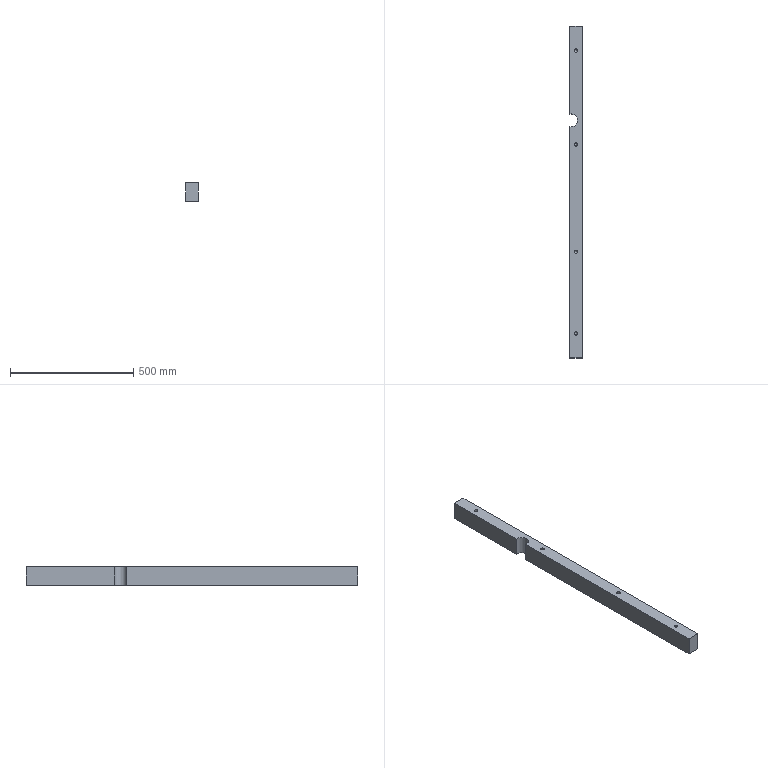Part | NX | features 3 2 | 1 solid | 24 faces | box 50 x 1345 x 75.5 mm | volume 4964830 mm3 | cylinder 9 | cone 8 | plane 7 | commonest cylinder face diameters 14.1 x8 52 x1
STEP:
#1=CARTESIAN_POINT('',(347.05,-572.5,256.5));
#2=VERTEX_POINT('',#1);
#3=CARTESIAN_POINT('',(340.,-572.5,256.5));
#4=DIRECTION('',(0.,0.,-1.));
#5=DIRECTION('',(1.,0.,0.));
#6=AXIS2_PLACEMENT_3D('',#3,#4,#5);
#7=CIRCLE('',#6,7.05);
#8=EDGE_CURVE('',#2,#2,#7,.T.);
#9=ORIENTED_EDGE('',*,*,#8,.T.);
#10=EDGE_LOOP('',(#9));
#11=FACE_BOUND('',#10,.T.);
#12=CARTESIAN_POINT('',(347.05,192.5,256.5));
#13=VERTEX_POINT('',#12);
#14=CARTESIAN_POINT('',(340.,192.5,256.5));
#15=DIRECTION('',(0.,0.,-1.));
#16=DIRECTION('',(1.,0.,0.));
#17=AXIS2_PLACEMENT_3D('',#14,#15,#16);
#18=CIRCLE('',#17,7.05);
#19=EDGE_CURVE('',#13,#13,#18,.T.);
#20=ORIENTED_EDGE('',*,*,#19,.T.);
#21=EDGE_LOOP('',(#20));
#22=FACE_BOUND('',#21,.T.);
#23=CARTESIAN_POINT('',(315.,315.515,256.5));
#24=VERTEX_POINT('',#23);
#25=CARTESIAN_POINT('',(315.,672.5,256.5));
#26=VERTEX_POINT('',#25);
#27=CARTESIAN_POINT('',(315.,193.,256.5));
#28=DIRECTION('',(0.,1.,0.));
#29=VECTOR('',#28,1000.);
#30=LINE('',#27,#29);
#31=EDGE_CURVE('',#24,#26,#30,.T.);
#32=ORIENTED_EDGE('',*,*,#31,.F.);
#33=CARTESIAN_POINT('',(315.,264.485,256.5));
#34=VERTEX_POINT('',#33);
#35=CARTESIAN_POINT('',(320.,290.,256.5));
#36=DIRECTION('',(0.,0.,1.));
#37=DIRECTION('',(1.,0.,0.));
#38=AXIS2_PLACEMENT_3D('',#35,#36,#37);
#39=CIRCLE('',#38,26.);
#40=EDGE_CURVE('',#34,#24,#39,.T.);
#41=ORIENTED_EDGE('',*,*,#40,.F.);
#42=CARTESIAN_POINT('',(315.,-672.5,256.5));
#43=VERTEX_POINT('',#42);
#44=CARTESIAN_POINT('',(315.,193.,256.5));
#45=DIRECTION('',(0.,1.,0.));
#46=VECTOR('',#45,1000.);
#47=LINE('',#44,#46);
#48=EDGE_CURVE('',#43,#34,#47,.T.);
#49=ORIENTED_EDGE('',*,*,#48,.F.);
#50=CARTESIAN_POINT('',(365.,-672.5,256.5));
#51=VERTEX_POINT('',#50);
#52=CARTESIAN_POINT('',(292.5,-672.5,256.5));
#53=DIRECTION('',(-1.,0.,0.));
#54=VECTOR('',#53,1000.);
#55=LINE('',#52,#54);
#56=EDGE_CURVE('',#51,#43,#55,.T.);
#57=ORIENTED_EDGE('',*,*,#56,.F.);
#58=CARTESIAN_POINT('',(365.,672.5,256.5));
#59=VERTEX_POINT('',#58);
#60=CARTESIAN_POINT('',(365.,193.,256.5));
#61=DIRECTION('',(0.,-1.,0.));
#62=VECTOR('',#61,1000.);
#63=LINE('',#60,#62);
#64=EDGE_CURVE('',#59,#51,#63,.T.);
#65=ORIENTED_EDGE('',*,*,#64,.F.);
#66=CARTESIAN_POINT('',(315.,672.5,256.5));
#67=DIRECTION('',(1.,0.,0.));
#68=VECTOR('',#67,1000.);
#69=LINE('',#66,#68);
#70=EDGE_CURVE('',#26,#59,#69,.T.);
#71=ORIENTED_EDGE('',*,*,#70,.F.);
#72=EDGE_LOOP('',(#32,#41,#49,#57,#65,#71));
#73=FACE_BOUND('',#72,.T.);
#74=CARTESIAN_POINT('',(347.05,572.5,256.5));
#75=VERTEX_POINT('',#74);
#76=CARTESIAN_POINT('',(340.,572.5,256.5));
#77=DIRECTION('',(0.,0.,-1.));
#78=DIRECTION('',(1.,0.,0.));
#79=AXIS2_PLACEMENT_3D('',#76,#77,#78);
#80=CIRCLE('',#79,7.05);
#81=EDGE_CURVE('',#75,#75,#80,.T.);
#82=ORIENTED_EDGE('',*,*,#81,.T.);
#83=EDGE_LOOP('',(#82));
#84=FACE_BOUND('',#83,.T.);
#85=CARTESIAN_POINT('',(347.05,-242.5,256.5));
#86=VERTEX_POINT('',#85);
#87=CARTESIAN_POINT('',(340.,-242.5,256.5));
#88=DIRECTION('',(0.,0.,-1.));
#89=DIRECTION('',(1.,0.,0.));
#90=AXIS2_PLACEMENT_3D('',#87,#88,#89);
#91=CIRCLE('',#90,7.05);
#92=EDGE_CURVE('',#86,#86,#91,.T.);
#93=ORIENTED_EDGE('',*,*,#92,.T.);
#94=EDGE_LOOP('',(#93));
#95=FACE_BOUND('',#94,.T.);
#96=CARTESIAN_POINT('',(2355.,0.,256.5));
#97=DIRECTION('',(0.,0.,1.));
#98=DIRECTION('',(-1.,0.,0.));
#99=AXIS2_PLACEMENT_3D('',#96,#97,#98);
#100=PLANE('',#99);
#101=ADVANCED_FACE('',(#11,#22,#73,#84,#95),#100,.T.);
#102=CARTESIAN_POINT('',(347.05,572.5,181.));
#103=VERTEX_POINT('',#102);
#104=CARTESIAN_POINT('',(340.,572.5,181.));
#105=DIRECTION('',(0.,0.,1.));
#106=DIRECTION('',(1.,0.,0.));
#107=AXIS2_PLACEMENT_3D('',#104,#105,#106);
#108=CIRCLE('',#107,7.05);
#109=EDGE_CURVE('',#103,#103,#108,.T.);
#110=ORIENTED_EDGE('',*,*,#109,.T.);
#111=EDGE_LOOP('',(#110));
#112=FACE_BOUND('',#111,.T.);
#113=CARTESIAN_POINT('',(347.05,-242.5,181.));
#114=VERTEX_POINT('',#113);
#115=CARTESIAN_POINT('',(340.,-242.5,181.));
#116=DIRECTION('',(0.,0.,1.));
#117=DIRECTION('',(1.,0.,0.));
#118=AXIS2_PLACEMENT_3D('',#115,#116,#117);
#119=CIRCLE('',#118,7.05);
#120=EDGE_CURVE('',#114,#114,#119,.T.);
#121=ORIENTED_EDGE('',*,*,#120,.T.);
#122=EDGE_LOOP('',(#121));
#123=FACE_BOUND('',#122,.T.);
#124=CARTESIAN_POINT('',(315.,264.485,181.));
#125=VERTEX_POINT('',#124);
#126=CARTESIAN_POINT('',(315.,-672.5,181.));
#127=VERTEX_POINT('',#126);
#128=CARTESIAN_POINT('',(315.,193.,181.));
#129=DIRECTION('',(0.,-1.,0.));
#130=VECTOR('',#129,1000.);
#131=LINE('',#128,#130);
#132=EDGE_CURVE('',#125,#127,#131,.T.);
#133=ORIENTED_EDGE('',*,*,#132,.F.);
#134=CARTESIAN_POINT('',(315.,315.515,181.));
#135=VERTEX_POINT('',#134);
#136=CARTESIAN_POINT('',(320.,290.,181.));
#137=DIRECTION('',(0.,0.,-1.));
#138=DIRECTION('',(-1.,0.,0.));
#139=AXIS2_PLACEMENT_3D('',#136,#137,#138);
#140=CIRCLE('',#139,26.);
#141=EDGE_CURVE('',#135,#125,#140,.T.);
#142=ORIENTED_EDGE('',*,*,#141,.F.);
#143=CARTESIAN_POINT('',(315.,672.5,181.));
#144=VERTEX_POINT('',#143);
#145=CARTESIAN_POINT('',(315.,193.,181.));
#146=DIRECTION('',(0.,-1.,0.));
#147=VECTOR('',#146,1000.);
#148=LINE('',#145,#147);
#149=EDGE_CURVE('',#144,#135,#148,.T.);
#150=ORIENTED_EDGE('',*,*,#149,.F.);
#151=CARTESIAN_POINT('',(365.,672.5,181.));
#152=VERTEX_POINT('',#151);
#153=CARTESIAN_POINT('',(1585.,672.5,181.));
#154=DIRECTION('',(1.,0.,0.));
#155=VECTOR('',#154,1000.);
#156=LINE('',#153,#155);
#157=EDGE_CURVE('',#144,#152,#156,.T.);
#158=ORIENTED_EDGE('',*,*,#157,.T.);
#159=CARTESIAN_POINT('',(365.,-672.5,181.));
#160=VERTEX_POINT('',#159);
#161=CARTESIAN_POINT('',(365.,193.,181.));
#162=DIRECTION('',(0.,1.,0.));
#163=VECTOR('',#162,1000.);
#164=LINE('',#161,#163);
#165=EDGE_CURVE('',#160,#152,#164,.T.);
#166=ORIENTED_EDGE('',*,*,#165,.F.);
#167=CARTESIAN_POINT('',(1585.,-672.5,181.));
#168=DIRECTION('',(-1.,0.,0.));
#169=VECTOR('',#168,1000.);
#170=LINE('',#167,#169);
#171=EDGE_CURVE('',#160,#127,#170,.T.);
#172=ORIENTED_EDGE('',*,*,#171,.T.);
#173=EDGE_LOOP('',(#133,#142,#150,#158,#166,#172));
#174=FACE_BOUND('',#173,.T.);
#175=CARTESIAN_POINT('',(347.05,-572.5,181.));
#176=VERTEX_POINT('',#175);
#177=CARTESIAN_POINT('',(340.,-572.5,181.));
#178=DIRECTION('',(0.,0.,1.));
#179=DIRECTION('',(1.,0.,0.));
#180=AXIS2_PLACEMENT_3D('',#177,#178,#179);
#181=CIRCLE('',#180,7.05);
#182=EDGE_CURVE('',#176,#176,#181,.T.);
#183=ORIENTED_EDGE('',*,*,#182,.T.);
#184=EDGE_LOOP('',(#183));
#185=FACE_BOUND('',#184,.T.);
#186=CARTESIAN_POINT('',(347.05,192.5,181.));
#187=VERTEX_POINT('',#186);
#188=CARTESIAN_POINT('',(340.,192.5,181.));
#189=DIRECTION('',(0.,0.,1.));
#190=DIRECTION('',(1.,0.,0.));
#191=AXIS2_PLACEMENT_3D('',#188,#189,#190);
#192=CIRCLE('',#191,7.05);
#193=EDGE_CURVE('',#187,#187,#192,.T.);
#194=ORIENTED_EDGE('',*,*,#193,.T.);
#195=EDGE_LOOP('',(#194));
#196=FACE_BOUND('',#195,.T.);
#197=CARTESIAN_POINT('',(1585.,193.,181.));
#198=DIRECTION('',(0.,0.,-1.));
#199=DIRECTION('',(-1.,0.,0.));
#200=AXIS2_PLACEMENT_3D('',#197,#198,#199);
#201=PLANE('',#200);
#202=ADVANCED_FACE('',(#112,#123,#174,#185,#196),#201,.T.);
#203=ORIENTED_EDGE('',*,*,#48,.T.);
#204=CARTESIAN_POINT('',(315.,264.485,218.75));
#205=DIRECTION('',(0.,0.,-1.));
#206=VECTOR('',#205,1000.);
#207=LINE('',#204,#206);
#208=EDGE_CURVE('',#34,#125,#207,.T.);
#209=ORIENTED_EDGE('',*,*,#208,.T.);
#210=ORIENTED_EDGE('',*,*,#132,.T.);
#211=CARTESIAN_POINT('',(315.,-672.5,-1.5));
#212=DIRECTION('',(0.,0.,1.));
#213=VECTOR('',#212,1000.);
#214=LINE('',#211,#213);
#215=EDGE_CURVE('',#127,#43,#214,.T.);
#216=ORIENTED_EDGE('',*,*,#215,.T.);
#217=EDGE_LOOP('',(#203,#209,#210,#216));
#218=FACE_BOUND('',#217,.T.);
#219=CARTESIAN_POINT('',(315.,193.,-1.5));
#220=DIRECTION('',(-1.,0.,0.));
#221=DIRECTION('',(0.,0.,-1.));
#222=AXIS2_PLACEMENT_3D('',#219,#220,#221);
#223=PLANE('',#222);
#224=ADVANCED_FACE('',(#218),#223,.T.);
#225=ORIENTED_EDGE('',*,*,#149,.T.);
#226=CARTESIAN_POINT('',(315.,315.515,218.75));
#227=DIRECTION('',(0.,0.,1.));
#228=VECTOR('',#227,1000.);
#229=LINE('',#226,#228);
#230=EDGE_CURVE('',#135,#24,#229,.T.);
#231=ORIENTED_EDGE('',*,*,#230,.T.);
#232=ORIENTED_EDGE('',*,*,#31,.T.);
#233=CARTESIAN_POINT('',(315.,672.5,-1.5));
#234=DIRECTION('',(0.,0.,-1.));
#235=VECTOR('',#234,1000.);
#236=LINE('',#233,#235);
#237=EDGE_CURVE('',#26,#144,#236,.T.);
#238=ORIENTED_EDGE('',*,*,#237,.T.);
#239=EDGE_LOOP('',(#225,#231,#232,#238));
#240=FACE_BOUND('',#239,.T.);
#241=CARTESIAN_POINT('',(315.,193.,-1.5));
#242=DIRECTION('',(-1.,0.,0.));
#243=DIRECTION('',(0.,0.,-1.));
#244=AXIS2_PLACEMENT_3D('',#241,#242,#243);
#245=PLANE('',#244);
#246=ADVANCED_FACE('',(#240),#245,.T.);
#247=CARTESIAN_POINT('',(365.,672.5,-1.5));
#248=DIRECTION('',(0.,0.,1.));
#249=VECTOR('',#248,1000.);
#250=LINE('',#247,#249);
#251=EDGE_CURVE('',#152,#59,#250,.T.);
#252=ORIENTED_EDGE('',*,*,#251,.T.);
#253=ORIENTED_EDGE('',*,*,#64,.T.);
#254=CARTESIAN_POINT('',(365.,-672.5,-1.5));
#255=DIRECTION('',(0.,0.,-1.));
#256=VECTOR('',#255,1000.);
#257=LINE('',#254,#256);
#258=EDGE_CURVE('',#51,#160,#257,.T.);
#259=ORIENTED_EDGE('',*,*,#258,.T.);
#260=ORIENTED_EDGE('',*,*,#165,.T.);
#261=EDGE_LOOP('',(#252,#253,#259,#260));
#262=FACE_BOUND('',#261,.T.);
#263=CARTESIAN_POINT('',(365.,193.,-1.5));
#264=DIRECTION('',(1.,0.,0.));
#265=DIRECTION('',(0.,0.,1.));
#266=AXIS2_PLACEMENT_3D('',#263,#264,#265);
#267=PLANE('',#266);
#268=ADVANCED_FACE('',(#262),#267,.T.);
#269=ORIENTED_EDGE('',*,*,#258,.F.);
#270=ORIENTED_EDGE('',*,*,#56,.T.);
#271=ORIENTED_EDGE('',*,*,#215,.F.);
#272=ORIENTED_EDGE('',*,*,#171,.F.);
#273=EDGE_LOOP('',(#269,#270,#271,#272));
#274=FACE_BOUND('',#273,.T.);
#275=CARTESIAN_POINT('',(292.5,-672.5,-103.));
#276=DIRECTION('',(0.,1.,0.));
#277=DIRECTION('',(1.,0.,0.));
#278=AXIS2_PLACEMENT_3D('',#275,#276,#277);
#279=PLANE('',#278);
#280=ADVANCED_FACE('',(#274),#279,.F.);
#281=ORIENTED_EDGE('',*,*,#237,.F.);
#282=ORIENTED_EDGE('',*,*,#70,.T.);
#283=ORIENTED_EDGE('',*,*,#251,.F.);
#284=ORIENTED_EDGE('',*,*,#157,.F.);
#285=EDGE_LOOP('',(#281,#282,#283,#284));
#286=FACE_BOUND('',#285,.T.);
#287=CARTESIAN_POINT('',(315.,672.5,231.5));
#288=DIRECTION('',(0.,1.,0.));
#289=DIRECTION('',(0.,0.,-1.));
#290=AXIS2_PLACEMENT_3D('',#287,#288,#289);
#291=PLANE('',#290);
#292=ADVANCED_FACE('',(#286),#291,.T.);
#293=ORIENTED_EDGE('',*,*,#40,.T.);
#294=ORIENTED_EDGE('',*,*,#230,.F.);
#295=ORIENTED_EDGE('',*,*,#141,.T.);
#296=ORIENTED_EDGE('',*,*,#208,.F.);
#297=EDGE_LOOP('',(#293,#294,#295,#296));
#298=FACE_BOUND('',#297,.T.);
#299=CARTESIAN_POINT('',(320.,290.,-261.5));
#300=DIRECTION('',(0.,0.,1.));
#301=DIRECTION('',(-1.,0.,0.));
#302=AXIS2_PLACEMENT_3D('',#299,#300,#301);
#303=CYLINDRICAL_SURFACE('',#302,26.);
#304=ADVANCED_FACE('',(#298),#303,.F.);
#305=ORIENTED_EDGE('',*,*,#120,.F.);
#306=EDGE_LOOP('',(#305));
#307=FACE_BOUND('',#306,.T.);
#308=CARTESIAN_POINT('',(347.05,-242.5,188.95));
#309=VERTEX_POINT('',#308);
#310=CARTESIAN_POINT('',(340.,-242.5,188.95));
#311=DIRECTION('',(0.,0.,-1.));
#312=DIRECTION('',(1.,0.,0.));
#313=AXIS2_PLACEMENT_3D('',#310,#311,#312);
#314=CIRCLE('',#313,7.05);
#315=EDGE_CURVE('',#309,#309,#314,.T.);
#316=ORIENTED_EDGE('',*,*,#315,.F.);
#317=EDGE_LOOP('',(#316));
#318=FACE_BOUND('',#317,.T.);
#319=CARTESIAN_POINT('',(340.,-242.5,181.));
#320=DIRECTION('',(0.,0.,1.));
#321=DIRECTION('',(-1.,0.,0.));
#322=AXIS2_PLACEMENT_3D('',#319,#320,#321);
#323=CYLINDRICAL_SURFACE('',#322,7.05);
#324=ADVANCED_FACE('',(#307,#318),#323,.F.);
#325=ORIENTED_EDGE('',*,*,#182,.F.);
#326=EDGE_LOOP('',(#325));
#327=FACE_BOUND('',#326,.T.);
#328=CARTESIAN_POINT('',(347.05,-572.5,188.95));
#329=VERTEX_POINT('',#328);
#330=CARTESIAN_POINT('',(340.,-572.5,188.95));
#331=DIRECTION('',(0.,0.,-1.));
#332=DIRECTION('',(1.,0.,0.));
#333=AXIS2_PLACEMENT_3D('',#330,#331,#332);
#334=CIRCLE('',#333,7.05);
#335=EDGE_CURVE('',#329,#329,#334,.T.);
#336=ORIENTED_EDGE('',*,*,#335,.F.);
#337=EDGE_LOOP('',(#336));
#338=FACE_BOUND('',#337,.T.);
#339=CARTESIAN_POINT('',(340.,-572.5,181.));
#340=DIRECTION('',(0.,0.,1.));
#341=DIRECTION('',(-1.,0.,0.));
#342=AXIS2_PLACEMENT_3D('',#339,#340,#341);
#343=CYLINDRICAL_SURFACE('',#342,7.05);
#344=ADVANCED_FACE('',(#327,#338),#343,.F.);
#345=ORIENTED_EDGE('',*,*,#109,.F.);
#346=EDGE_LOOP('',(#345));
#347=FACE_BOUND('',#346,.T.);
#348=CARTESIAN_POINT('',(347.05,572.5,188.95));
#349=VERTEX_POINT('',#348);
#350=CARTESIAN_POINT('',(340.,572.5,188.95));
#351=DIRECTION('',(0.,0.,-1.));
#352=DIRECTION('',(1.,0.,0.));
#353=AXIS2_PLACEMENT_3D('',#350,#351,#352);
#354=CIRCLE('',#353,7.05);
#355=EDGE_CURVE('',#349,#349,#354,.T.);
#356=ORIENTED_EDGE('',*,*,#355,.F.);
#357=EDGE_LOOP('',(#356));
#358=FACE_BOUND('',#357,.T.);
#359=CARTESIAN_POINT('',(340.,572.5,181.));
#360=DIRECTION('',(0.,0.,1.));
#361=DIRECTION('',(-1.,0.,0.));
#362=AXIS2_PLACEMENT_3D('',#359,#360,#361);
#363=CYLINDRICAL_SURFACE('',#362,7.05);
#364=ADVANCED_FACE('',(#347,#358),#363,.F.);
#365=ORIENTED_EDGE('',*,*,#193,.F.);
#366=EDGE_LOOP('',(#365));
#367=FACE_BOUND('',#366,.T.);
#368=CARTESIAN_POINT('',(347.05,192.5,188.95));
#369=VERTEX_POINT('',#368);
#370=CARTESIAN_POINT('',(340.,192.5,188.95));
#371=DIRECTION('',(0.,0.,-1.));
#372=DIRECTION('',(1.,0.,0.));
#373=AXIS2_PLACEMENT_3D('',#370,#371,#372);
#374=CIRCLE('',#373,7.05);
#375=EDGE_CURVE('',#369,#369,#374,.T.);
#376=ORIENTED_EDGE('',*,*,#375,.F.);
#377=EDGE_LOOP('',(#376));
#378=FACE_BOUND('',#377,.T.);
#379=CARTESIAN_POINT('',(340.,192.5,181.));
#380=DIRECTION('',(0.,0.,1.));
#381=DIRECTION('',(-1.,0.,0.));
#382=AXIS2_PLACEMENT_3D('',#379,#380,#381);
#383=CYLINDRICAL_SURFACE('',#382,7.05);
#384=ADVANCED_FACE('',(#367,#378),#383,.F.);
#385=CARTESIAN_POINT('',(340.,-242.5,196.));
#386=VERTEX_POINT('',#385);
#387=VERTEX_LOOP('',#386);
#388=FACE_BOUND('',#387,.T.);
#389=ORIENTED_EDGE('',*,*,#315,.T.);
#390=EDGE_LOOP('',(#389));
#391=FACE_BOUND('',#390,.T.);
#392=CARTESIAN_POINT('',(340.,-242.5,188.95));
#393=DIRECTION('',(0.,0.,-1.));
#394=DIRECTION('',(1.,0.,0.));
#395=AXIS2_PLACEMENT_3D('',#392,#393,#394);
#396=CONICAL_SURFACE('',#395,7.05,0.7854);
#397=ADVANCED_FACE('',(#388,#391),#396,.F.);
#398=CARTESIAN_POINT('',(340.,-572.5,196.));
#399=VERTEX_POINT('',#398);
#400=VERTEX_LOOP('',#399);
#401=FACE_BOUND('',#400,.T.);
#402=ORIENTED_EDGE('',*,*,#335,.T.);
#403=EDGE_LOOP('',(#402));
#404=FACE_BOUND('',#403,.T.);
#405=CARTESIAN_POINT('',(340.,-572.5,188.95));
#406=DIRECTION('',(0.,0.,-1.));
#407=DIRECTION('',(1.,0.,0.));
#408=AXIS2_PLACEMENT_3D('',#405,#406,#407);
#409=CONICAL_SURFACE('',#408,7.05,0.7854);
#410=ADVANCED_FACE('',(#401,#404),#409,.F.);
#411=CARTESIAN_POINT('',(340.,572.5,196.));
#412=VERTEX_POINT('',#411);
#413=VERTEX_LOOP('',#412);
#414=FACE_BOUND('',#413,.T.);
#415=ORIENTED_EDGE('',*,*,#355,.T.);
#416=EDGE_LOOP('',(#415));
#417=FACE_BOUND('',#416,.T.);
#418=CARTESIAN_POINT('',(340.,572.5,188.95));
#419=DIRECTION('',(0.,0.,-1.));
#420=DIRECTION('',(1.,0.,0.));
#421=AXIS2_PLACEMENT_3D('',#418,#419,#420);
#422=CONICAL_SURFACE('',#421,7.05,0.7854);
#423=ADVANCED_FACE('',(#414,#417),#422,.F.);
#424=CARTESIAN_POINT('',(340.,192.5,196.));
#425=VERTEX_POINT('',#424);
#426=VERTEX_LOOP('',#425);
#427=FACE_BOUND('',#426,.T.);
#428=ORIENTED_EDGE('',*,*,#375,.T.);
#429=EDGE_LOOP('',(#428));
#430=FACE_BOUND('',#429,.T.);
#431=CARTESIAN_POINT('',(340.,192.5,188.95));
#432=DIRECTION('',(0.,0.,-1.));
#433=DIRECTION('',(1.,0.,0.));
#434=AXIS2_PLACEMENT_3D('',#431,#432,#433);
#435=CONICAL_SURFACE('',#434,7.05,0.7854);
#436=ADVANCED_FACE('',(#427,#430),#435,.F.);
#437=CARTESIAN_POINT('',(332.95,192.5,248.55));
#438=VERTEX_POINT('',#437);
#439=CARTESIAN_POINT('',(340.,192.5,248.55));
#440=DIRECTION('',(0.,0.,-1.));
#441=DIRECTION('',(-1.,0.,0.));
#442=AXIS2_PLACEMENT_3D('',#439,#440,#441);
#443=CIRCLE('',#442,7.05);
#444=EDGE_CURVE('',#438,#438,#443,.T.);
#445=ORIENTED_EDGE('',*,*,#444,.T.);
#446=EDGE_LOOP('',(#445));
#447=FACE_BOUND('',#446,.T.);
#448=ORIENTED_EDGE('',*,*,#19,.F.);
#449=EDGE_LOOP('',(#448));
#450=FACE_BOUND('',#449,.T.);
#451=CARTESIAN_POINT('',(340.,192.5,256.5));
#452=DIRECTION('',(0.,0.,-1.));
#453=DIRECTION('',(-1.,0.,0.));
#454=AXIS2_PLACEMENT_3D('',#451,#452,#453);
#455=CYLINDRICAL_SURFACE('',#454,7.05);
#456=ADVANCED_FACE('',(#447,#450),#455,.F.);
#457=CARTESIAN_POINT('',(340.,192.5,241.5));
#458=VERTEX_POINT('',#457);
#459=VERTEX_LOOP('',#458);
#460=FACE_BOUND('',#459,.T.);
#461=ORIENTED_EDGE('',*,*,#444,.F.);
#462=EDGE_LOOP('',(#461));
#463=FACE_BOUND('',#462,.T.);
#464=CARTESIAN_POINT('',(340.,192.5,248.55));
#465=DIRECTION('',(0.,0.,1.));
#466=DIRECTION('',(-1.,0.,0.));
#467=AXIS2_PLACEMENT_3D('',#464,#465,#466);
#468=CONICAL_SURFACE('',#467,7.05,0.7854);
#469=ADVANCED_FACE('',(#460,#463),#468,.F.);
#470=CARTESIAN_POINT('',(332.95,572.5,248.55));
#471=VERTEX_POINT('',#470);
#472=CARTESIAN_POINT('',(340.,572.5,248.55));
#473=DIRECTION('',(0.,0.,-1.));
#474=DIRECTION('',(-1.,0.,0.));
#475=AXIS2_PLACEMENT_3D('',#472,#473,#474);
#476=CIRCLE('',#475,7.05);
#477=EDGE_CURVE('',#471,#471,#476,.T.);
#478=ORIENTED_EDGE('',*,*,#477,.T.);
#479=EDGE_LOOP('',(#478));
#480=FACE_BOUND('',#479,.T.);
#481=ORIENTED_EDGE('',*,*,#81,.F.);
#482=EDGE_LOOP('',(#481));
#483=FACE_BOUND('',#482,.T.);
#484=CARTESIAN_POINT('',(340.,572.5,256.5));
#485=DIRECTION('',(0.,0.,-1.));
#486=DIRECTION('',(-1.,0.,0.));
#487=AXIS2_PLACEMENT_3D('',#484,#485,#486);
#488=CYLINDRICAL_SURFACE('',#487,7.05);
#489=ADVANCED_FACE('',(#480,#483),#488,.F.);
#490=CARTESIAN_POINT('',(340.,572.5,241.5));
#491=VERTEX_POINT('',#490);
#492=VERTEX_LOOP('',#491);
#493=FACE_BOUND('',#492,.T.);
#494=ORIENTED_EDGE('',*,*,#477,.F.);
#495=EDGE_LOOP('',(#494));
#496=FACE_BOUND('',#495,.T.);
#497=CARTESIAN_POINT('',(340.,572.5,248.55));
#498=DIRECTION('',(0.,0.,1.));
#499=DIRECTION('',(-1.,0.,0.));
#500=AXIS2_PLACEMENT_3D('',#497,#498,#499);
#501=CONICAL_SURFACE('',#500,7.05,0.7854);
#502=ADVANCED_FACE('',(#493,#496),#501,.F.);
#503=CARTESIAN_POINT('',(332.95,-572.5,248.55));
#504=VERTEX_POINT('',#503);
#505=CARTESIAN_POINT('',(340.,-572.5,248.55));
#506=DIRECTION('',(0.,0.,-1.));
#507=DIRECTION('',(-1.,0.,0.));
#508=AXIS2_PLACEMENT_3D('',#505,#506,#507);
#509=CIRCLE('',#508,7.05);
#510=EDGE_CURVE('',#504,#504,#509,.T.);
#511=ORIENTED_EDGE('',*,*,#510,.T.);
#512=EDGE_LOOP('',(#511));
#513=FACE_BOUND('',#512,.T.);
#514=ORIENTED_EDGE('',*,*,#8,.F.);
#515=EDGE_LOOP('',(#514));
#516=FACE_BOUND('',#515,.T.);
#517=CARTESIAN_POINT('',(340.,-572.5,256.5));
#518=DIRECTION('',(0.,0.,-1.));
#519=DIRECTION('',(-1.,0.,0.));
#520=AXIS2_PLACEMENT_3D('',#517,#518,#519);
#521=CYLINDRICAL_SURFACE('',#520,7.05);
#522=ADVANCED_FACE('',(#513,#516),#521,.F.);
#523=CARTESIAN_POINT('',(340.,-572.5,241.5));
#524=VERTEX_POINT('',#523);
#525=VERTEX_LOOP('',#524);
#526=FACE_BOUND('',#525,.T.);
#527=ORIENTED_EDGE('',*,*,#510,.F.);
#528=EDGE_LOOP('',(#527));
#529=FACE_BOUND('',#528,.T.);
#530=CARTESIAN_POINT('',(340.,-572.5,248.55));
#531=DIRECTION('',(0.,0.,1.));
#532=DIRECTION('',(-1.,0.,0.));
#533=AXIS2_PLACEMENT_3D('',#530,#531,#532);
#534=CONICAL_SURFACE('',#533,7.05,0.7854);
#535=ADVANCED_FACE('',(#526,#529),#534,.F.);
#536=CARTESIAN_POINT('',(332.95,-242.5,248.55));
#537=VERTEX_POINT('',#536);
#538=CARTESIAN_POINT('',(340.,-242.5,248.55));
#539=DIRECTION('',(0.,0.,-1.));
#540=DIRECTION('',(-1.,0.,0.));
#541=AXIS2_PLACEMENT_3D('',#538,#539,#540);
#542=CIRCLE('',#541,7.05);
#543=EDGE_CURVE('',#537,#537,#542,.T.);
#544=ORIENTED_EDGE('',*,*,#543,.T.);
#545=EDGE_LOOP('',(#544));
#546=FACE_BOUND('',#545,.T.);
#547=ORIENTED_EDGE('',*,*,#92,.F.);
#548=EDGE_LOOP('',(#547));
#549=FACE_BOUND('',#548,.T.);
#550=CARTESIAN_POINT('',(340.,-242.5,256.5));
#551=DIRECTION('',(0.,0.,-1.));
#552=DIRECTION('',(-1.,0.,0.));
#553=AXIS2_PLACEMENT_3D('',#550,#551,#552);
#554=CYLINDRICAL_SURFACE('',#553,7.05);
#555=ADVANCED_FACE('',(#546,#549),#554,.F.);
#556=CARTESIAN_POINT('',(340.,-242.5,241.5));
#557=VERTEX_POINT('',#556);
#558=VERTEX_LOOP('',#557);
#559=FACE_BOUND('',#558,.T.);
#560=ORIENTED_EDGE('',*,*,#543,.F.);
#561=EDGE_LOOP('',(#560));
#562=FACE_BOUND('',#561,.T.);
#563=CARTESIAN_POINT('',(340.,-242.5,248.55));
#564=DIRECTION('',(0.,0.,1.));
#565=DIRECTION('',(-1.,0.,0.));
#566=AXIS2_PLACEMENT_3D('',#563,#564,#565);
#567=CONICAL_SURFACE('',#566,7.05,0.7854);
#568=ADVANCED_FACE('',(#559,#562),#567,.F.);
#569=CLOSED_SHELL('',(#101,#202,#224,#246,#268,#280,#292,#304,#324,#344,#364,#384,#397,#410,#423,#436,#456,#469,#489,#502,#522,#535,#555,#568));
#570=MANIFOLD_SOLID_BREP('',#569);
#571=(LENGTH_UNIT()NAMED_UNIT(*)SI_UNIT(.MILLI.,.METRE.));
#572=UNCERTAINTY_MEASURE_WITH_UNIT(LENGTH_MEASURE(0.00001),#571,'','');
#573=(NAMED_UNIT(*)PLANE_ANGLE_UNIT()SI_UNIT($,.RADIAN.));
#574=(NAMED_UNIT(*)SI_UNIT($,.STERADIAN.)SOLID_ANGLE_UNIT());
#575=(GEOMETRIC_REPRESENTATION_CONTEXT(3)GLOBAL_UNCERTAINTY_ASSIGNED_CONTEXT((#572))GLOBAL_UNIT_ASSIGNED_CONTEXT((#571,#573,#574))REPRESENTATION_CONTEXT('',''));
#576=ADVANCED_BREP_SHAPE_REPRESENTATION('',(#570),#575);